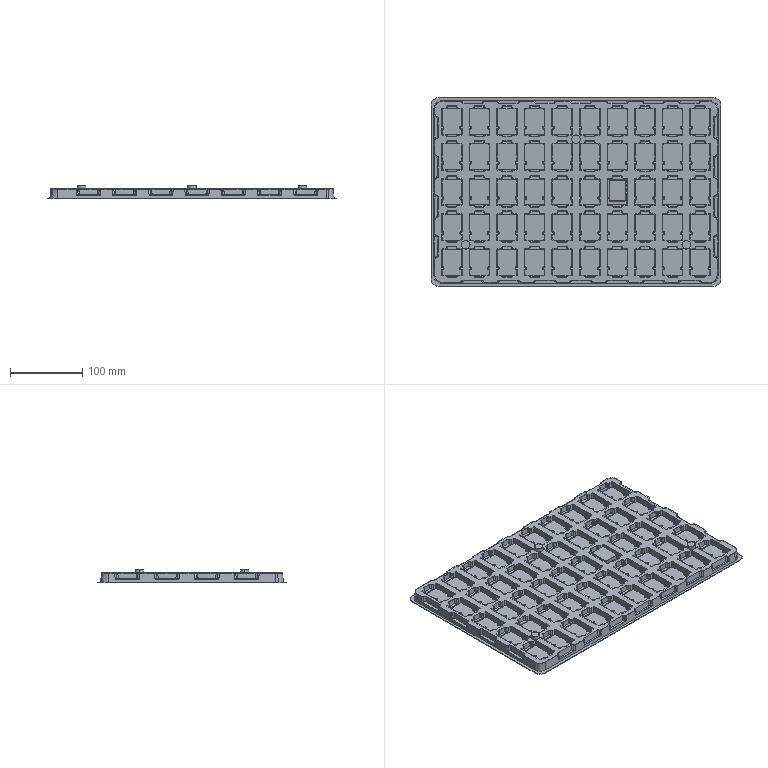Part | STEP file | 11-Xpptp-tu-3d-2c11 | 2 solids | 4362 faces | volume 141535 mm3 | cylinder 2200 | plane 2134 | cone 16 | spline 12 | commonest cylinder face diameters 3 x444 2.4 x400 4 x400 4.6 x244 1 x212 1.4 x200